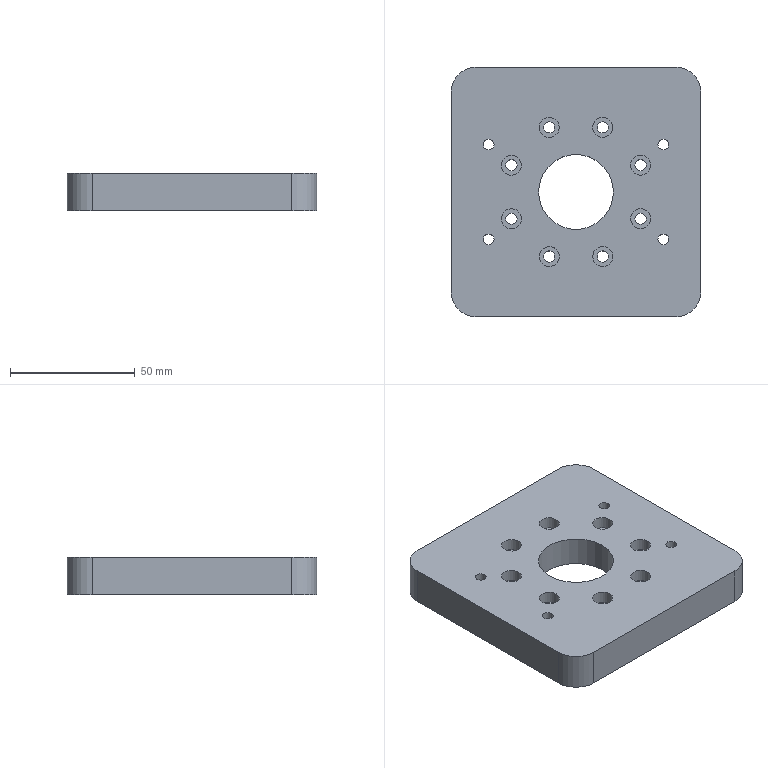NC program | NX | posted with a generic post | part box 100 x 100 x 15 mm
Lines 1753 to 2115 of 2115:
(DRILLING , TOOL : D6A45)
N3480 T07 M6
N3482 G54
N3484 G17 G0 G90 X0. Y0. S5000 M3
N3486 G43 Z30. H7
N3488 G94 G81 G98 Z-1. F250. R3.
N3490 X25.869 Y10.715
N3492 X35. Y19.
N3494 X10.715 Y25.869
N3496 X-10.715
N3498 X-35. Y19.
N3500 X-25.869 Y10.715
N3502 Y-10.715
N3504 X-35. Y-19.
N3506 X-10.715 Y-25.869
N3508 X10.715
N3510 X25.869 Y-10.715
N3512 X35. Y-19.
N3514 G80
N3516 G0 X35. Y-19. Z30.
N3518 M5
(DRILLING_COPY , TOOL : 4.3ZT)
N3520 T14 M6
N3522 G54
N3524 G17 G0 G90 X35. Y19. S2000 M3
N3526 G43 Z30. H14
N3528 G94 G83 G98 Z-17.792 F250. Q2. R3.
N3530 Y-19.
N3532 X-35.
N3534 Y19.
N3536 G80
N3538 G0 X-35. Y19. Z30.
N3540 M5
(DRILLING_COPY_COPY , TOOL : 4.5ZT)
N3542 T15 M6
N3544 G54
N3546 G17 G0 G90 X10.715 Y-25.869 S2000 M3
N3548 G43 Z30. H15
N3550 G94 G83 G98 Z-16.352 F250. Q2. R3.
N3552 X-10.715
N3554 X-25.869 Y-10.715
N3556 Y10.715
N3558 X-10.715 Y25.869
N3560 X10.715
N3562 X25.869 Y10.715
N3564 Y-10.715
N3566 G80
N3568 G0 X25.869 Y-10.715 Z30.
N3570 M5
(HOLE_MILLING_1 , TOOL : D6)
N3572 T06 M6
N3574 G54
N3576 G17 G0 G90 X-25.869 Y-10.715 S9500 M3
N3578 G43 Z30. H6
N3580 Z0.5
N3582 G94 G3 X-25.369 Y-11.215 R0.5 F1500.
N3584 X-24.869 Y-10.715 R0.5
N3586 X-24.869 Y-10.715 Z0. I-1. J0.
N3588 X-24.869 Y-10.715 Z-0.5 I-1. J0.
N3590 X-24.869 Y-10.715 Z-1. I-1. J0.
N3592 X-24.869 Y-10.715 Z-1.5 I-1. J0.
N3594 X-24.869 Y-10.715 Z-2. I-1. J0.
N3596 X-24.869 Y-10.715 Z-2.5 I-1. J0.
N3598 X-24.869 Y-10.715 Z-3. I-1. J0.
N3600 X-24.869 Y-10.715 Z-3.5 I-1. J0.
N3602 X-24.869 Y-10.715 Z-4. I-1. J0.
N3604 X-24.869 Y-10.715 Z-4.5 I-1. J0.
N3606 X-24.869 Y-10.715 Z-5. I-1. J0.
N3608 X-25.869 Y-9.715 R1.
N3610 X-24.869 Y-10.715 R-1.
N3612 X-25.369 Y-10.215 R0.5
N3614 X-25.869 Y-10.715 R0.5
N3616 G0 Z30.
N3618 Y10.715
N3620 Z0.5
N3622 G3 X-25.369 Y10.215 R0.5
N3624 X-24.869 Y10.715 R0.5
N3626 X-24.869 Y10.715 Z0. I-1. J0.
N3628 X-24.869 Y10.715 Z-0.5 I-1. J0.
N3630 X-24.869 Y10.715 Z-1. I-1. J0.
N3632 X-24.869 Y10.715 Z-1.5 I-1. J0.
N3634 X-24.869 Y10.715 Z-2. I-1. J0.
N3636 X-24.869 Y10.715 Z-2.5 I-1. J0.
N3638 X-24.869 Y10.715 Z-3. I-1. J0.
N3640 X-24.869 Y10.715 Z-3.5 I-1. J0.
N3642 X-24.869 Y10.715 Z-4. I-1. J0.
N3644 X-24.869 Y10.715 Z-4.5 I-1. J0.
N3646 X-24.869 Y10.715 Z-5. I-1. J0.
N3648 X-25.869 Y11.715 R1.
N3650 X-24.869 Y10.715 R-1.
N3652 X-25.369 Y11.215 R0.5
N3654 X-25.869 Y10.715 R0.5
N3656 G0 Z30.
N3658 X-10.715 Y25.869
N3660 Z0.5
N3662 G3 X-10.215 Y25.369 R0.5
N3664 X-9.715 Y25.869 R0.5
N3666 X-9.715 Y25.869 Z0. I-1. J0.
N3668 X-9.715 Y25.869 Z-0.5 I-1. J0.
N3670 X-9.715 Y25.869 Z-1. I-1. J0.
N3672 X-9.715 Y25.869 Z-1.5 I-1. J0.
N3674 X-9.715 Y25.869 Z-2. I-1. J0.
N3676 X-9.715 Y25.869 Z-2.5 I-1. J0.
N3678 X-9.715 Y25.869 Z-3. I-1. J0.
N3680 X-9.715 Y25.869 Z-3.5 I-1. J0.
N3682 X-9.715 Y25.869 Z-4. I-1. J0.
N3684 X-9.715 Y25.869 Z-4.5 I-1. J0.
N3686 X-9.715 Y25.869 Z-5. I-1. J0.
N3688 X-10.715 Y26.869 R1.
N3690 X-9.715 Y25.869 R-1.
N3692 X-10.215 Y26.369 R0.5
N3694 X-10.715 Y25.869 R0.5
N3696 G0 Z30.
N3698 X10.715
N3700 Z0.5
N3702 G3 X11.215 Y25.369 R0.5
N3704 X11.715 Y25.869 R0.5
N3706 X11.715 Y25.869 Z0. I-1. J0.
N3708 X11.715 Y25.869 Z-0.5 I-1. J0.
N3710 X11.715 Y25.869 Z-1. I-1. J0.
N3712 X11.715 Y25.869 Z-1.5 I-1. J0.
N3714 X11.715 Y25.869 Z-2. I-1. J0.
N3716 X11.715 Y25.869 Z-2.5 I-1. J0.
N3718 X11.715 Y25.869 Z-3. I-1. J0.
N3720 X11.715 Y25.869 Z-3.5 I-1. J0.
N3722 X11.715 Y25.869 Z-4. I-1. J0.
N3724 X11.715 Y25.869 Z-4.5 I-1. J0.
N3726 X11.715 Y25.869 Z-5. I-1. J0.
N3728 X10.715 Y26.869 R1.
N3730 X11.715 Y25.869 R-1.
N3732 X11.215 Y26.369 R0.5
N3734 X10.715 Y25.869 R0.5
N3736 G0 Z30.
N3738 X25.869 Y10.715
N3740 Z0.5
N3742 G3 X26.369 Y10.215 R0.5
N3744 X26.869 Y10.715 R0.5
N3746 X26.869 Y10.715 Z0. I-1. J0.
N3748 X26.869 Y10.715 Z-0.5 I-1. J0.
N3750 X26.869 Y10.715 Z-1. I-1. J0.
N3752 X26.869 Y10.715 Z-1.5 I-1. J0.
N3754 X26.869 Y10.715 Z-2. I-1. J0.
N3756 X26.869 Y10.715 Z-2.5 I-1. J0.
N3758 X26.869 Y10.715 Z-3. I-1. J0.
N3760 X26.869 Y10.715 Z-3.5 I-1. J0.
N3762 X26.869 Y10.715 Z-4. I-1. J0.
N3764 X26.869 Y10.715 Z-4.5 I-1. J0.
N3766 X26.869 Y10.715 Z-5. I-1. J0.
N3768 X25.869 Y11.715 R1.
N3770 X26.869 Y10.715 R-1.
N3772 X26.369 Y11.215 R0.5
N3774 X25.869 Y10.715 R0.5
N3776 G0 Z30.
N3778 Y-10.715
N3780 Z0.5
N3782 G3 X26.369 Y-11.215 R0.5
N3784 X26.869 Y-10.715 R0.5
N3786 X26.869 Y-10.715 Z0. I-1. J0.
N3788 X26.869 Y-10.715 Z-0.5 I-1. J0.
N3790 X26.869 Y-10.715 Z-1. I-1. J0.
N3792 X26.869 Y-10.715 Z-1.5 I-1. J0.
N3794 X26.869 Y-10.715 Z-2. I-1. J0.
N3796 X26.869 Y-10.715 Z-2.5 I-1. J0.
N3798 X26.869 Y-10.715 Z-3. I-1. J0.
N3800 X26.869 Y-10.715 Z-3.5 I-1. J0.
N3802 X26.869 Y-10.715 Z-4. I-1. J0.
N3804 X26.869 Y-10.715 Z-4.5 I-1. J0.
N3806 X26.869 Y-10.715 Z-5. I-1. J0.
N3808 X25.869 Y-9.715 R1.
N3810 X26.869 Y-10.715 R-1.
N3812 X26.369 Y-10.215 R0.5
N3814 X25.869 Y-10.715 R0.5
N3816 G0 Z30.
N3818 X10.715 Y-25.869
N3820 Z0.5
N3822 G3 X11.215 Y-26.369 R0.5
N3824 X11.715 Y-25.869 R0.5
N3826 X11.715 Y-25.869 Z0. I-1. J0.
N3828 X11.715 Y-25.869 Z-0.5 I-1. J0.
N3830 X11.715 Y-25.869 Z-1. I-1. J0.
N3832 X11.715 Y-25.869 Z-1.5 I-1. J0.
N3834 X11.715 Y-25.869 Z-2. I-1. J0.
N3836 X11.715 Y-25.869 Z-2.5 I-1. J0.
N3838 X11.715 Y-25.869 Z-3. I-1. J0.
N3840 X11.715 Y-25.869 Z-3.5 I-1. J0.
N3842 X11.715 Y-25.869 Z-4. I-1. J0.
N3844 X11.715 Y-25.869 Z-4.5 I-1. J0.
N3846 X11.715 Y-25.869 Z-5. I-1. J0.
N3848 X10.715 Y-24.869 R1.
N3850 X11.715 Y-25.869 R-1.
N3852 X11.215 Y-25.369 R0.5
N3854 X10.715 Y-25.869 R0.5
N3856 G0 Z30.
N3858 X-10.715
N3860 Z0.5
N3862 G3 X-10.215 Y-26.369 R0.5
N3864 X-9.715 Y-25.869 R0.5
N3866 X-9.715 Y-25.869 Z0. I-1. J0.
N3868 X-9.715 Y-25.869 Z-0.5 I-1. J0.
N3870 X-9.715 Y-25.869 Z-1. I-1. J0.
N3872 X-9.715 Y-25.869 Z-1.5 I-1. J0.
N3874 X-9.715 Y-25.869 Z-2. I-1. J0.
N3876 X-9.715 Y-25.869 Z-2.5 I-1. J0.
N3878 X-9.715 Y-25.869 Z-3. I-1. J0.
N3880 X-9.715 Y-25.869 Z-3.5 I-1. J0.
N3882 X-9.715 Y-25.869 Z-4. I-1. J0.
N3884 X-9.715 Y-25.869 Z-4.5 I-1. J0.
N3886 X-9.715 Y-25.869 Z-5. I-1. J0.
N3888 X-10.715 Y-24.869 R1.
N3890 X-9.715 Y-25.869 R-1.
N3892 X-10.215 Y-25.369 R0.5
N3894 X-10.715 Y-25.869 R0.5
N3896 G0 Z30.
N3898 M5
(PLANAR_MILL , TOOL : D6A45)
N3900 T07 M6
N3902 G54
N3904 G17 G0 G90 X-35.75 Y19.866 S9500 M3
N3906 G43 Z30. H7
N3908 Z0.5
N3910 G94 G1 Z-1. F1250.
N3912 G3 X-36.25 Y19. R1.
N3914 X-35. Y17.75 R1.25
N3916 X-36.25 Y19. R-1.25
N3918 X-35.75 Y18.134 R1.
N3920 G1 Z0.5
N3922 G0 Z30.
N3924 X-28.469 Y11.581
N3926 Z0.5
N3928 G1 Z-1.
N3930 G3 X-28.969 Y10.715 R1.
N3932 X-25.869 Y7.615 R3.1
N3934 X-28.969 Y10.715 R-3.1
N3936 X-28.469 Y9.849 R1.
N3938 G1 Z0.5
N3940 G0 Z30.
N3942 X-9.849 Y28.469
N3944 Z0.5
N3946 G1 Z-1.
N3948 G3 X-10.715 Y28.969 R1.
N3950 X-13.815 Y25.869 R3.1
N3952 X-10.715 Y28.969 R-3.1
N3954 X-11.581 Y28.469 R1.
N3956 G1 Z0.5
N3958 G0 Z30.
N3960 X11.581
N3962 Z0.5
N3964 G1 Z-1.
N3966 G3 X10.715 Y28.969 R1.
N3968 X7.615 Y25.869 R3.1
N3970 X10.715 Y28.969 R-3.1
N3972 X9.849 Y28.469 R1.
N3974 G1 Z0.5
N3976 G0 Z30.
N3978 X35.75 Y18.134
N3980 Z0.5
N3982 G1 Z-1.
N3984 G3 X36.25 Y19. R1.
N3986 X35. Y20.25 R1.25
N3988 X36.25 Y19. R-1.25
N3990 X35.75 Y19.866 R1.
N3992 G1 Z0.5
N3994 G0 Z30.
N3996 X28.469 Y9.849
N3998 Z0.5
N4000 G1 Z-1.
N4002 G3 X28.969 Y10.715 R1.
N4004 X25.869 Y13.815 R3.1
N4006 X28.969 Y10.715 R-3.1
N4008 X28.469 Y11.581 R1.
N4010 G1 Z0.5
N4012 G0 Z30.
N4014 Y-11.581
N4016 Z0.5
N4018 G1 Z-1.
N4020 G3 X28.969 Y-10.715 R1.
N4022 X25.869 Y-7.615 R3.1
N4024 X28.969 Y-10.715 R-3.1
N4026 X28.469 Y-9.849 R1.
N4028 G1 Z0.5
N4030 G0 Z30.
N4032 X35.75 Y-19.866
N4034 Z0.5
N4036 G1 Z-1.
N4038 G3 X36.25 Y-19. R1.
N4040 X35. Y-17.75 R1.25
N4042 X36.25 Y-19. R-1.25
N4044 X35.75 Y-18.134 R1.
N4046 G1 Z0.5
N4048 G0 Z30.
N4050 X9.849 Y-28.469
N4052 Z0.5
N4054 G1 Z-1.
N4056 G3 X10.715 Y-28.969 R1.
N4058 X13.815 Y-25.869 R3.1
N4060 X10.715 Y-28.969 R-3.1
N4062 X11.581 Y-28.469 R1.
N4064 G1 Z0.5
N4066 G0 Z30.
N4068 X-11.581
N4070 Z0.5
N4072 G1 Z-1.
N4074 G3 X-10.715 Y-28.969 R1.
N4076 X-7.615 Y-25.869 R3.1
N4078 X-10.715 Y-28.969 R-3.1
N4080 X-9.849 Y-28.469 R1.
N4082 G1 Z0.5
N4084 G0 Z30.
N4086 X-35.75 Y-18.134
N4088 Z0.5
N4090 G1 Z-1.
N4092 G3 X-36.25 Y-19. R1.
N4094 X-35. Y-20.25 R1.25
N4096 X-36.25 Y-19. R-1.25
N4098 X-35.75 Y-19.866 R1.
N4100 G1 Z0.5
N4102 G0 Z30.
N4104 X-28.469 Y-9.849
N4106 Z0.5
N4108 G1 Z-1.
N4110 G3 X-28.969 Y-10.715 R1.
N4112 X-25.869 Y-13.815 R3.1
N4114 X-28.969 Y-10.715 R-3.1
N4116 X-28.469 Y-11.581 R1.
N4118 G1 Z0.5
N4120 G0 Z30.
N4122 X-51.4 Y-0.866
N4124 Z0.5
N4126 G1 Z-1.
N4128 G3 X-50.9 Y0. R1.
N4130 G1 Y40.
N4132 G2 X-40. Y50.9 R10.9
N4134 G1 X40.
N4136 G2 X50.9 Y40. R10.9
N4138 G1 Y-40.
N4140 G2 X40. Y-50.9 R10.9
N4142 G1 X-40.
N4144 G2 X-50.9 Y-40. R10.9
N4146 G1 Y0.
N4148 G3 X-51.4 Y0.866 R1.
N4150 G1 Z0.5
N4152 G0 Z30.
N4154 X-13.6
N4156 Z0.5
N4158 G1 Z-1.
N4160 G3 X-14.1 Y0. R1.
N4162 X0. Y-14.1 R14.1
N4164 X-14.1 Y0. R-14.1
N4166 X-13.6 Y-0.866 R1.
N4168 G1 Z0.5
N4170 G0 Z30.
N4172 M5
N4174 M2